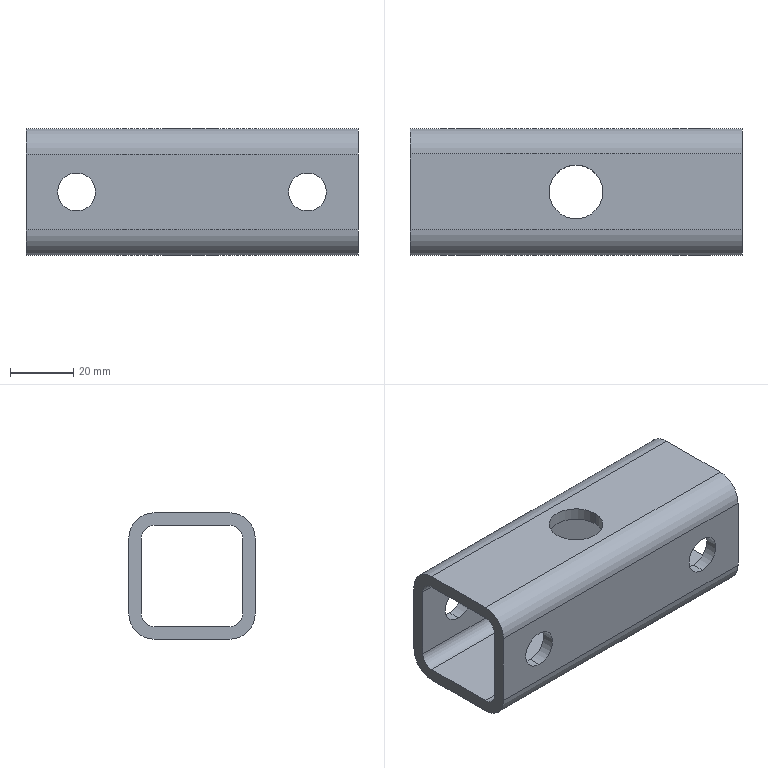Part | SolidWorks | features HoleWzd 1, ICE 1, WeldMemberFeat 1, WeldmentFeature 1 | 1 solid | 30 faces | box 105 x 40 x 40 mm | volume 52528 mm3 | cylinder 20 | plane 10 | commonest cylinder face diameters 12 x8 8 x4 16 x4 17 x4
STEP:
#1=CARTESIAN_POINT('',(44.,0.,20.));
#2=VERTEX_POINT('',#1);
#3=CARTESIAN_POINT('',(61.,0.,20.));
#4=VERTEX_POINT('',#3);
#5=CARTESIAN_POINT('',(52.5,0.,20.));
#6=DIRECTION('',(0.,0.,1.));
#7=DIRECTION('',(-1.,0.,0.));
#8=AXIS2_PLACEMENT_3D('',#5,#6,#7);
#9=CIRCLE('',#8,8.5);
#10=EDGE_CURVE('',#2,#4,#9,.T.);
#11=ORIENTED_EDGE('',*,*,#10,.T.);
#12=CARTESIAN_POINT('',(61.,0.,16.));
#13=VERTEX_POINT('',#12);
#14=CARTESIAN_POINT('',(61.,0.,44.042));
#15=DIRECTION('',(0.,0.,-1.));
#16=VECTOR('',#15,1000.);
#17=LINE('',#14,#16);
#18=EDGE_CURVE('',#4,#13,#17,.T.);
#19=ORIENTED_EDGE('',*,*,#18,.T.);
#20=CARTESIAN_POINT('',(44.,0.,16.));
#21=VERTEX_POINT('',#20);
#22=CARTESIAN_POINT('',(52.5,0.,16.));
#23=DIRECTION('',(0.,0.,-1.));
#24=DIRECTION('',(-1.,0.,0.));
#25=AXIS2_PLACEMENT_3D('',#22,#23,#24);
#26=CIRCLE('',#25,8.5);
#27=EDGE_CURVE('',#13,#21,#26,.T.);
#28=ORIENTED_EDGE('',*,*,#27,.T.);
#29=CARTESIAN_POINT('',(44.,0.,44.042));
#30=DIRECTION('',(0.,0.,-1.));
#31=VECTOR('',#30,1000.);
#32=LINE('',#29,#31);
#33=EDGE_CURVE('',#2,#21,#32,.T.);
#34=ORIENTED_EDGE('',*,*,#33,.F.);
#35=EDGE_LOOP('',(#11,#19,#28,#34));
#36=FACE_OUTER_BOUND('',#35,.T.);
#37=CARTESIAN_POINT('',(52.5,0.,44.042));
#38=DIRECTION('',(0.,0.,-1.));
#39=DIRECTION('',(-1.,0.,0.));
#40=AXIS2_PLACEMENT_3D('',#37,#38,#39);
#41=CYLINDRICAL_SURFACE('',#40,8.5);
#42=ADVANCED_FACE('',(#36),#41,.F.);
#43=CARTESIAN_POINT('',(44.,0.,-16.));
#44=VERTEX_POINT('',#43);
#45=CARTESIAN_POINT('',(61.,0.,-16.));
#46=VERTEX_POINT('',#45);
#47=CARTESIAN_POINT('',(52.5,0.,-16.));
#48=DIRECTION('',(0.,0.,1.));
#49=DIRECTION('',(1.,0.,0.));
#50=AXIS2_PLACEMENT_3D('',#47,#48,#49);
#51=CIRCLE('',#50,8.5);
#52=EDGE_CURVE('',#44,#46,#51,.T.);
#53=ORIENTED_EDGE('',*,*,#52,.T.);
#54=CARTESIAN_POINT('',(61.,0.,-20.));
#55=VERTEX_POINT('',#54);
#56=CARTESIAN_POINT('',(61.,0.,44.042));
#57=DIRECTION('',(0.,0.,-1.));
#58=VECTOR('',#57,1000.);
#59=LINE('',#56,#58);
#60=EDGE_CURVE('',#46,#55,#59,.T.);
#61=ORIENTED_EDGE('',*,*,#60,.T.);
#62=CARTESIAN_POINT('',(44.,0.,-20.));
#63=VERTEX_POINT('',#62);
#64=CARTESIAN_POINT('',(52.5,0.,-20.));
#65=DIRECTION('',(0.,0.,-1.));
#66=DIRECTION('',(-1.,0.,0.));
#67=AXIS2_PLACEMENT_3D('',#64,#65,#66);
#68=CIRCLE('',#67,8.5);
#69=EDGE_CURVE('',#55,#63,#68,.T.);
#70=ORIENTED_EDGE('',*,*,#69,.T.);
#71=CARTESIAN_POINT('',(44.,0.,44.042));
#72=DIRECTION('',(0.,0.,-1.));
#73=VECTOR('',#72,1000.);
#74=LINE('',#71,#73);
#75=EDGE_CURVE('',#44,#63,#74,.T.);
#76=ORIENTED_EDGE('',*,*,#75,.F.);
#77=EDGE_LOOP('',(#53,#61,#70,#76));
#78=FACE_OUTER_BOUND('',#77,.T.);
#79=CARTESIAN_POINT('',(52.5,0.,44.042));
#80=DIRECTION('',(0.,0.,-1.));
#81=DIRECTION('',(-1.,0.,0.));
#82=AXIS2_PLACEMENT_3D('',#79,#80,#81);
#83=CYLINDRICAL_SURFACE('',#82,8.5);
#84=ADVANCED_FACE('',(#78),#83,.F.);
#85=CARTESIAN_POINT('',(16.,-20.,-6.));
#86=VERTEX_POINT('',#85);
#87=CARTESIAN_POINT('',(16.,-20.,6.));
#88=VERTEX_POINT('',#87);
#89=CARTESIAN_POINT('',(16.,-20.,0.));
#90=DIRECTION('',(0.,1.,0.));
#91=DIRECTION('',(0.,0.,1.));
#92=AXIS2_PLACEMENT_3D('',#89,#90,#91);
#93=CIRCLE('',#92,6.);
#94=EDGE_CURVE('',#86,#88,#93,.T.);
#95=ORIENTED_EDGE('',*,*,#94,.F.);
#96=CARTESIAN_POINT('',(16.,-16.,-6.));
#97=VERTEX_POINT('',#96);
#98=CARTESIAN_POINT('',(16.,20.,-6.));
#99=DIRECTION('',(0.,1.,0.));
#100=VECTOR('',#99,1000.);
#101=LINE('',#98,#100);
#102=EDGE_CURVE('',#86,#97,#101,.T.);
#103=ORIENTED_EDGE('',*,*,#102,.T.);
#104=CARTESIAN_POINT('',(16.,-16.,6.));
#105=VERTEX_POINT('',#104);
#106=CARTESIAN_POINT('',(16.,-16.,0.));
#107=DIRECTION('',(0.,1.,0.));
#108=DIRECTION('',(0.,0.,1.));
#109=AXIS2_PLACEMENT_3D('',#106,#107,#108);
#110=CIRCLE('',#109,6.);
#111=EDGE_CURVE('',#97,#105,#110,.T.);
#112=ORIENTED_EDGE('',*,*,#111,.T.);
#113=CARTESIAN_POINT('',(16.,20.,6.));
#114=DIRECTION('',(0.,1.,0.));
#115=VECTOR('',#114,1000.);
#116=LINE('',#113,#115);
#117=EDGE_CURVE('',#88,#105,#116,.T.);
#118=ORIENTED_EDGE('',*,*,#117,.F.);
#119=EDGE_LOOP('',(#95,#103,#112,#118));
#120=FACE_OUTER_BOUND('',#119,.T.);
#121=CARTESIAN_POINT('',(16.,20.,0.));
#122=DIRECTION('',(0.,1.,0.));
#123=DIRECTION('',(0.,0.,1.));
#124=AXIS2_PLACEMENT_3D('',#121,#122,#123);
#125=CYLINDRICAL_SURFACE('',#124,6.);
#126=ADVANCED_FACE('',(#120),#125,.F.);
#127=CARTESIAN_POINT('',(16.,16.,6.));
#128=VERTEX_POINT('',#127);
#129=CARTESIAN_POINT('',(16.,16.,-6.));
#130=VERTEX_POINT('',#129);
#131=CARTESIAN_POINT('',(16.,16.,0.));
#132=DIRECTION('',(0.,-1.,0.));
#133=DIRECTION('',(0.,0.,-1.));
#134=AXIS2_PLACEMENT_3D('',#131,#132,#133);
#135=CIRCLE('',#134,6.);
#136=EDGE_CURVE('',#128,#130,#135,.T.);
#137=ORIENTED_EDGE('',*,*,#136,.T.);
#138=CARTESIAN_POINT('',(16.,20.,-6.));
#139=VERTEX_POINT('',#138);
#140=CARTESIAN_POINT('',(16.,20.,-6.));
#141=DIRECTION('',(0.,1.,0.));
#142=VECTOR('',#141,1000.);
#143=LINE('',#140,#142);
#144=EDGE_CURVE('',#130,#139,#143,.T.);
#145=ORIENTED_EDGE('',*,*,#144,.T.);
#146=CARTESIAN_POINT('',(16.,20.,6.));
#147=VERTEX_POINT('',#146);
#148=CARTESIAN_POINT('',(16.,20.,0.));
#149=DIRECTION('',(0.,1.,0.));
#150=DIRECTION('',(0.,0.,1.));
#151=AXIS2_PLACEMENT_3D('',#148,#149,#150);
#152=CIRCLE('',#151,6.);
#153=EDGE_CURVE('',#139,#147,#152,.T.);
#154=ORIENTED_EDGE('',*,*,#153,.T.);
#155=CARTESIAN_POINT('',(16.,20.,6.));
#156=DIRECTION('',(0.,1.,0.));
#157=VECTOR('',#156,1000.);
#158=LINE('',#155,#157);
#159=EDGE_CURVE('',#128,#147,#158,.T.);
#160=ORIENTED_EDGE('',*,*,#159,.F.);
#161=EDGE_LOOP('',(#137,#145,#154,#160));
#162=FACE_OUTER_BOUND('',#161,.T.);
#163=CARTESIAN_POINT('',(16.,20.,0.));
#164=DIRECTION('',(0.,1.,0.));
#165=DIRECTION('',(0.,0.,1.));
#166=AXIS2_PLACEMENT_3D('',#163,#164,#165);
#167=CYLINDRICAL_SURFACE('',#166,6.);
#168=ADVANCED_FACE('',(#162),#167,.F.);
#169=CARTESIAN_POINT('',(89.,-20.,-6.));
#170=VERTEX_POINT('',#169);
#171=CARTESIAN_POINT('',(89.,-20.,6.));
#172=VERTEX_POINT('',#171);
#173=CARTESIAN_POINT('',(89.,-20.,0.));
#174=DIRECTION('',(0.,1.,0.));
#175=DIRECTION('',(0.,0.,1.));
#176=AXIS2_PLACEMENT_3D('',#173,#174,#175);
#177=CIRCLE('',#176,6.);
#178=EDGE_CURVE('',#170,#172,#177,.T.);
#179=ORIENTED_EDGE('',*,*,#178,.F.);
#180=CARTESIAN_POINT('',(89.,-16.,-6.));
#181=VERTEX_POINT('',#180);
#182=CARTESIAN_POINT('',(89.,20.,-6.));
#183=DIRECTION('',(0.,1.,0.));
#184=VECTOR('',#183,1000.);
#185=LINE('',#182,#184);
#186=EDGE_CURVE('',#170,#181,#185,.T.);
#187=ORIENTED_EDGE('',*,*,#186,.T.);
#188=CARTESIAN_POINT('',(89.,-16.,6.));
#189=VERTEX_POINT('',#188);
#190=CARTESIAN_POINT('',(89.,-16.,0.));
#191=DIRECTION('',(0.,1.,0.));
#192=DIRECTION('',(0.,0.,1.));
#193=AXIS2_PLACEMENT_3D('',#190,#191,#192);
#194=CIRCLE('',#193,6.);
#195=EDGE_CURVE('',#181,#189,#194,.T.);
#196=ORIENTED_EDGE('',*,*,#195,.T.);
#197=CARTESIAN_POINT('',(89.,20.,6.));
#198=DIRECTION('',(0.,1.,0.));
#199=VECTOR('',#198,1000.);
#200=LINE('',#197,#199);
#201=EDGE_CURVE('',#172,#189,#200,.T.);
#202=ORIENTED_EDGE('',*,*,#201,.F.);
#203=EDGE_LOOP('',(#179,#187,#196,#202));
#204=FACE_OUTER_BOUND('',#203,.T.);
#205=CARTESIAN_POINT('',(89.,20.,0.));
#206=DIRECTION('',(0.,1.,0.));
#207=DIRECTION('',(0.,0.,1.));
#208=AXIS2_PLACEMENT_3D('',#205,#206,#207);
#209=CYLINDRICAL_SURFACE('',#208,6.);
#210=ADVANCED_FACE('',(#204),#209,.F.);
#211=CARTESIAN_POINT('',(89.,16.,6.));
#212=VERTEX_POINT('',#211);
#213=CARTESIAN_POINT('',(89.,16.,-6.));
#214=VERTEX_POINT('',#213);
#215=CARTESIAN_POINT('',(89.,16.,0.));
#216=DIRECTION('',(0.,-1.,0.));
#217=DIRECTION('',(0.,0.,-1.));
#218=AXIS2_PLACEMENT_3D('',#215,#216,#217);
#219=CIRCLE('',#218,6.);
#220=EDGE_CURVE('',#212,#214,#219,.T.);
#221=ORIENTED_EDGE('',*,*,#220,.T.);
#222=CARTESIAN_POINT('',(89.,20.,-6.));
#223=VERTEX_POINT('',#222);
#224=CARTESIAN_POINT('',(89.,20.,-6.));
#225=DIRECTION('',(0.,1.,0.));
#226=VECTOR('',#225,1000.);
#227=LINE('',#224,#226);
#228=EDGE_CURVE('',#214,#223,#227,.T.);
#229=ORIENTED_EDGE('',*,*,#228,.T.);
#230=CARTESIAN_POINT('',(89.,20.,6.));
#231=VERTEX_POINT('',#230);
#232=CARTESIAN_POINT('',(89.,20.,0.));
#233=DIRECTION('',(0.,1.,0.));
#234=DIRECTION('',(0.,0.,1.));
#235=AXIS2_PLACEMENT_3D('',#232,#233,#234);
#236=CIRCLE('',#235,6.);
#237=EDGE_CURVE('',#223,#231,#236,.T.);
#238=ORIENTED_EDGE('',*,*,#237,.T.);
#239=CARTESIAN_POINT('',(89.,20.,6.));
#240=DIRECTION('',(0.,1.,0.));
#241=VECTOR('',#240,1000.);
#242=LINE('',#239,#241);
#243=EDGE_CURVE('',#212,#231,#242,.T.);
#244=ORIENTED_EDGE('',*,*,#243,.F.);
#245=EDGE_LOOP('',(#221,#229,#238,#244));
#246=FACE_OUTER_BOUND('',#245,.T.);
#247=CARTESIAN_POINT('',(89.,20.,0.));
#248=DIRECTION('',(0.,1.,0.));
#249=DIRECTION('',(0.,0.,1.));
#250=AXIS2_PLACEMENT_3D('',#247,#248,#249);
#251=CYLINDRICAL_SURFACE('',#250,6.);
#252=ADVANCED_FACE('',(#246),#251,.F.);
#253=CARTESIAN_POINT('',(0.,20.,12.));
#254=VERTEX_POINT('',#253);
#255=CARTESIAN_POINT('',(0.,12.,20.));
#256=VERTEX_POINT('',#255);
#257=CARTESIAN_POINT('',(0.,12.,12.));
#258=DIRECTION('',(1.,0.,0.));
#259=DIRECTION('',(0.,0.,-1.));
#260=AXIS2_PLACEMENT_3D('',#257,#258,#259);
#261=CIRCLE('',#260,8.);
#262=EDGE_CURVE('',#254,#256,#261,.T.);
#263=ORIENTED_EDGE('',*,*,#262,.T.);
#264=CARTESIAN_POINT('',(105.,12.,20.));
#265=VERTEX_POINT('',#264);
#266=CARTESIAN_POINT('',(105.,12.,20.));
#267=DIRECTION('',(-1.,0.,0.));
#268=VECTOR('',#267,1000.);
#269=LINE('',#266,#268);
#270=EDGE_CURVE('',#265,#256,#269,.T.);
#271=ORIENTED_EDGE('',*,*,#270,.F.);
#272=CARTESIAN_POINT('',(105.,20.,12.));
#273=VERTEX_POINT('',#272);
#274=CARTESIAN_POINT('',(105.,12.,12.));
#275=DIRECTION('',(1.,0.,0.));
#276=DIRECTION('',(0.,0.,-1.));
#277=AXIS2_PLACEMENT_3D('',#274,#275,#276);
#278=CIRCLE('',#277,8.);
#279=EDGE_CURVE('',#273,#265,#278,.T.);
#280=ORIENTED_EDGE('',*,*,#279,.F.);
#281=CARTESIAN_POINT('',(105.,20.,12.));
#282=DIRECTION('',(-1.,0.,0.));
#283=VECTOR('',#282,1000.);
#284=LINE('',#281,#283);
#285=EDGE_CURVE('',#273,#254,#284,.T.);
#286=ORIENTED_EDGE('',*,*,#285,.T.);
#287=EDGE_LOOP('',(#263,#271,#280,#286));
#288=FACE_OUTER_BOUND('',#287,.T.);
#289=CARTESIAN_POINT('',(105.,12.,12.));
#290=DIRECTION('',(-1.,0.,0.));
#291=DIRECTION('',(0.,0.,1.));
#292=AXIS2_PLACEMENT_3D('',#289,#290,#291);
#293=CYLINDRICAL_SURFACE('',#292,8.);
#294=ADVANCED_FACE('',(#288),#293,.T.);
#295=ORIENTED_EDGE('',*,*,#10,.F.);
#296=CARTESIAN_POINT('',(52.5,0.,20.));
#297=DIRECTION('',(0.,0.,1.));
#298=DIRECTION('',(-1.,0.,0.));
#299=AXIS2_PLACEMENT_3D('',#296,#297,#298);
#300=CIRCLE('',#299,8.5);
#301=EDGE_CURVE('',#4,#2,#300,.T.);
#302=ORIENTED_EDGE('',*,*,#301,.F.);
#303=EDGE_LOOP('',(#295,#302));
#304=FACE_BOUND('',#303,.T.);
#305=CARTESIAN_POINT('',(0.,-12.,20.));
#306=VERTEX_POINT('',#305);
#307=CARTESIAN_POINT('',(0.,12.,20.));
#308=DIRECTION('',(0.,-1.,0.));
#309=VECTOR('',#308,1000.);
#310=LINE('',#307,#309);
#311=EDGE_CURVE('',#256,#306,#310,.T.);
#312=ORIENTED_EDGE('',*,*,#311,.T.);
#313=CARTESIAN_POINT('',(105.,-12.,20.));
#314=VERTEX_POINT('',#313);
#315=CARTESIAN_POINT('',(105.,-12.,20.));
#316=DIRECTION('',(-1.,0.,0.));
#317=VECTOR('',#316,1000.);
#318=LINE('',#315,#317);
#319=EDGE_CURVE('',#314,#306,#318,.T.);
#320=ORIENTED_EDGE('',*,*,#319,.F.);
#321=CARTESIAN_POINT('',(105.,12.,20.));
#322=DIRECTION('',(0.,-1.,0.));
#323=VECTOR('',#322,1000.);
#324=LINE('',#321,#323);
#325=EDGE_CURVE('',#265,#314,#324,.T.);
#326=ORIENTED_EDGE('',*,*,#325,.F.);
#327=ORIENTED_EDGE('',*,*,#270,.T.);
#328=EDGE_LOOP('',(#312,#320,#326,#327));
#329=FACE_OUTER_BOUND('',#328,.T.);
#330=CARTESIAN_POINT('',(105.,12.,20.));
#331=DIRECTION('',(0.,0.,-1.));
#332=DIRECTION('',(-1.,0.,0.));
#333=AXIS2_PLACEMENT_3D('',#330,#331,#332);
#334=PLANE('',#333);
#335=ADVANCED_FACE('',(#304,#329),#334,.F.);
#336=CARTESIAN_POINT('',(0.,-20.,12.));
#337=VERTEX_POINT('',#336);
#338=CARTESIAN_POINT('',(0.,-12.,12.));
#339=DIRECTION('',(1.,0.,0.));
#340=DIRECTION('',(0.,0.,-1.));
#341=AXIS2_PLACEMENT_3D('',#338,#339,#340);
#342=CIRCLE('',#341,8.);
#343=EDGE_CURVE('',#306,#337,#342,.T.);
#344=ORIENTED_EDGE('',*,*,#343,.T.);
#345=CARTESIAN_POINT('',(105.,-20.,12.));
#346=VERTEX_POINT('',#345);
#347=CARTESIAN_POINT('',(105.,-20.,12.));
#348=DIRECTION('',(-1.,0.,0.));
#349=VECTOR('',#348,1000.);
#350=LINE('',#347,#349);
#351=EDGE_CURVE('',#346,#337,#350,.T.);
#352=ORIENTED_EDGE('',*,*,#351,.F.);
#353=CARTESIAN_POINT('',(105.,-12.,12.));
#354=DIRECTION('',(1.,0.,0.));
#355=DIRECTION('',(0.,0.,-1.));
#356=AXIS2_PLACEMENT_3D('',#353,#354,#355);
#357=CIRCLE('',#356,8.);
#358=EDGE_CURVE('',#314,#346,#357,.T.);
#359=ORIENTED_EDGE('',*,*,#358,.F.);
#360=ORIENTED_EDGE('',*,*,#319,.T.);
#361=EDGE_LOOP('',(#344,#352,#359,#360));
#362=FACE_OUTER_BOUND('',#361,.T.);
#363=CARTESIAN_POINT('',(105.,-12.,12.));
#364=DIRECTION('',(-1.,0.,0.));
#365=DIRECTION('',(0.,0.,1.));
#366=AXIS2_PLACEMENT_3D('',#363,#364,#365);
#367=CYLINDRICAL_SURFACE('',#366,8.);
#368=ADVANCED_FACE('',(#362),#367,.T.);
#369=CARTESIAN_POINT('',(16.,-20.,0.));
#370=DIRECTION('',(0.,1.,0.));
#371=DIRECTION('',(0.,0.,1.));
#372=AXIS2_PLACEMENT_3D('',#369,#370,#371);
#373=CIRCLE('',#372,6.);
#374=EDGE_CURVE('',#88,#86,#373,.T.);
#375=ORIENTED_EDGE('',*,*,#374,.T.);
#376=ORIENTED_EDGE('',*,*,#94,.T.);
#377=EDGE_LOOP('',(#375,#376));
#378=FACE_BOUND('',#377,.T.);
#379=CARTESIAN_POINT('',(89.,-20.,0.));
#380=DIRECTION('',(0.,1.,0.));
#381=DIRECTION('',(0.,0.,1.));
#382=AXIS2_PLACEMENT_3D('',#379,#380,#381);
#383=CIRCLE('',#382,6.);
#384=EDGE_CURVE('',#172,#170,#383,.T.);
#385=ORIENTED_EDGE('',*,*,#384,.T.);
#386=ORIENTED_EDGE('',*,*,#178,.T.);
#387=EDGE_LOOP('',(#385,#386));
#388=FACE_BOUND('',#387,.T.);
#389=CARTESIAN_POINT('',(0.,-20.,-12.));
#390=VERTEX_POINT('',#389);
#391=CARTESIAN_POINT('',(0.,-20.,-12.));
#392=DIRECTION('',(0.,0.,-1.));
#393=VECTOR('',#392,1000.);
#394=LINE('',#391,#393);
#395=EDGE_CURVE('',#337,#390,#394,.T.);
#396=ORIENTED_EDGE('',*,*,#395,.T.);
#397=CARTESIAN_POINT('',(105.,-20.,-12.));
#398=VERTEX_POINT('',#397);
#399=CARTESIAN_POINT('',(105.,-20.,-12.));
#400=DIRECTION('',(-1.,0.,0.));
#401=VECTOR('',#400,1000.);
#402=LINE('',#399,#401);
#403=EDGE_CURVE('',#398,#390,#402,.T.);
#404=ORIENTED_EDGE('',*,*,#403,.F.);
#405=CARTESIAN_POINT('',(105.,-20.,-12.));
#406=DIRECTION('',(0.,0.,-1.));
#407=VECTOR('',#406,1000.);
#408=LINE('',#405,#407);
#409=EDGE_CURVE('',#346,#398,#408,.T.);
#410=ORIENTED_EDGE('',*,*,#409,.F.);
#411=ORIENTED_EDGE('',*,*,#351,.T.);
#412=EDGE_LOOP('',(#396,#404,#410,#411));
#413=FACE_OUTER_BOUND('',#412,.T.);
#414=CARTESIAN_POINT('',(105.,-20.,-12.));
#415=DIRECTION('',(0.,1.,0.));
#416=DIRECTION('',(0.,0.,1.));
#417=AXIS2_PLACEMENT_3D('',#414,#415,#416);
#418=PLANE('',#417);
#419=ADVANCED_FACE('',(#378,#388,#413),#418,.F.);
#420=CARTESIAN_POINT('',(0.,-12.,-20.));
#421=VERTEX_POINT('',#420);
#422=CARTESIAN_POINT('',(0.,-12.,-12.));
#423=DIRECTION('',(1.,0.,0.));
#424=DIRECTION('',(0.,0.,-1.));
#425=AXIS2_PLACEMENT_3D('',#422,#423,#424);
#426=CIRCLE('',#425,8.);
#427=EDGE_CURVE('',#390,#421,#426,.T.);
#428=ORIENTED_EDGE('',*,*,#427,.T.);
#429=CARTESIAN_POINT('',(105.,-12.,-20.));
#430=VERTEX_POINT('',#429);
#431=CARTESIAN_POINT('',(105.,-12.,-20.));
#432=DIRECTION('',(-1.,0.,0.));
#433=VECTOR('',#432,1000.);
#434=LINE('',#431,#433);
#435=EDGE_CURVE('',#430,#421,#434,.T.);
#436=ORIENTED_EDGE('',*,*,#435,.F.);
#437=CARTESIAN_POINT('',(105.,-12.,-12.));
#438=DIRECTION('',(1.,0.,0.));
#439=DIRECTION('',(0.,0.,-1.));
#440=AXIS2_PLACEMENT_3D('',#437,#438,#439);
#441=CIRCLE('',#440,8.);
#442=EDGE_CURVE('',#398,#430,#441,.T.);
#443=ORIENTED_EDGE('',*,*,#442,.F.);
#444=ORIENTED_EDGE('',*,*,#403,.T.);
#445=EDGE_LOOP('',(#428,#436,#443,#444));
#446=FACE_OUTER_BOUND('',#445,.T.);
#447=CARTESIAN_POINT('',(105.,-12.,-12.));
#448=DIRECTION('',(-1.,0.,0.));
#449=DIRECTION('',(0.,0.,1.));
#450=AXIS2_PLACEMENT_3D('',#447,#448,#449);
#451=CYLINDRICAL_SURFACE('',#450,8.);
#452=ADVANCED_FACE('',(#446),#451,.T.);
#453=CARTESIAN_POINT('',(52.5,0.,-20.));
#454=DIRECTION('',(0.,0.,-1.));
#455=DIRECTION('',(-1.,0.,0.));
#456=AXIS2_PLACEMENT_3D('',#453,#454,#455);
#457=CIRCLE('',#456,8.5);
#458=EDGE_CURVE('',#63,#55,#457,.T.);
#459=ORIENTED_EDGE('',*,*,#458,.F.);
#460=ORIENTED_EDGE('',*,*,#69,.F.);
#461=EDGE_LOOP('',(#459,#460));
#462=FACE_BOUND('',#461,.T.);
#463=CARTESIAN_POINT('',(0.,12.,-20.));
#464=VERTEX_POINT('',#463);
#465=CARTESIAN_POINT('',(0.,-12.,-20.));
#466=DIRECTION('',(0.,1.,0.));
#467=VECTOR('',#466,1000.);
#468=LINE('',#465,#467);
#469=EDGE_CURVE('',#421,#464,#468,.T.);
#470=ORIENTED_EDGE('',*,*,#469,.T.);
#471=CARTESIAN_POINT('',(105.,12.,-20.));
#472=VERTEX_POINT('',#471);
#473=CARTESIAN_POINT('',(105.,12.,-20.));
#474=DIRECTION('',(-1.,0.,0.));
#475=VECTOR('',#474,1000.);
#476=LINE('',#473,#475);
#477=EDGE_CURVE('',#472,#464,#476,.T.);
#478=ORIENTED_EDGE('',*,*,#477,.F.);
#479=CARTESIAN_POINT('',(105.,-12.,-20.));
#480=DIRECTION('',(0.,1.,0.));
#481=VECTOR('',#480,1000.);
#482=LINE('',#479,#481);
#483=EDGE_CURVE('',#430,#472,#482,.T.);
#484=ORIENTED_EDGE('',*,*,#483,.F.);
#485=ORIENTED_EDGE('',*,*,#435,.T.);
#486=EDGE_LOOP('',(#470,#478,#484,#485));
#487=FACE_OUTER_BOUND('',#486,.T.);
#488=CARTESIAN_POINT('',(105.,-12.,-20.));
#489=DIRECTION('',(0.,0.,1.));
#490=DIRECTION('',(1.,0.,0.));
#491=AXIS2_PLACEMENT_3D('',#488,#489,#490);
#492=PLANE('',#491);
#493=ADVANCED_FACE('',(#462,#487),#492,.F.);
#494=CARTESIAN_POINT('',(0.,20.,-12.));
#495=VERTEX_POINT('',#494);
#496=CARTESIAN_POINT('',(0.,12.,-12.));
#497=DIRECTION('',(1.,0.,0.));
#498=DIRECTION('',(0.,0.,-1.));
#499=AXIS2_PLACEMENT_3D('',#496,#497,#498);
#500=CIRCLE('',#499,8.);
#501=EDGE_CURVE('',#464,#495,#500,.T.);
#502=ORIENTED_EDGE('',*,*,#501,.T.);
#503=CARTESIAN_POINT('',(105.,20.,-12.));
#504=VERTEX_POINT('',#503);
#505=CARTESIAN_POINT('',(105.,20.,-12.));
#506=DIRECTION('',(-1.,0.,0.));
#507=VECTOR('',#506,1000.);
#508=LINE('',#505,#507);
#509=EDGE_CURVE('',#504,#495,#508,.T.);
#510=ORIENTED_EDGE('',*,*,#509,.F.);
#511=CARTESIAN_POINT('',(105.,12.,-12.));
#512=DIRECTION('',(1.,0.,0.));
#513=DIRECTION('',(0.,0.,-1.));
#514=AXIS2_PLACEMENT_3D('',#511,#512,#513);
#515=CIRCLE('',#514,8.);
#516=EDGE_CURVE('',#472,#504,#515,.T.);
#517=ORIENTED_EDGE('',*,*,#516,.F.);
#518=ORIENTED_EDGE('',*,*,#477,.T.);
#519=EDGE_LOOP('',(#502,#510,#517,#518));
#520=FACE_OUTER_BOUND('',#519,.T.);
#521=CARTESIAN_POINT('',(105.,12.,-12.));
#522=DIRECTION('',(-1.,0.,0.));
#523=DIRECTION('',(0.,0.,1.));
#524=AXIS2_PLACEMENT_3D('',#521,#522,#523);
#525=CYLINDRICAL_SURFACE('',#524,8.);
#526=ADVANCED_FACE('',(#520),#525,.T.);
#527=CARTESIAN_POINT('',(0.,-12.,16.));
#528=VERTEX_POINT('',#527);
#529=CARTESIAN_POINT('',(0.,-16.,12.));
#530=VERTEX_POINT('',#529);
#531=CARTESIAN_POINT('',(0.,-12.,12.));
#532=DIRECTION('',(1.,0.,0.));
#533=DIRECTION('',(0.,0.,-1.));
#534=AXIS2_PLACEMENT_3D('',#531,#532,#533);
#535=CIRCLE('',#534,4.);
#536=EDGE_CURVE('',#528,#530,#535,.T.);
#537=ORIENTED_EDGE('',*,*,#536,.F.);
#538=CARTESIAN_POINT('',(105.,-12.,16.));
#539=VERTEX_POINT('',#538);
#540=CARTESIAN_POINT('',(105.,-12.,16.));
#541=DIRECTION('',(-1.,0.,0.));
#542=VECTOR('',#541,1000.);
#543=LINE('',#540,#542);
#544=EDGE_CURVE('',#539,#528,#543,.T.);
#545=ORIENTED_EDGE('',*,*,#544,.F.);
#546=CARTESIAN_POINT('',(105.,-16.,12.));
#547=VERTEX_POINT('',#546);
#548=CARTESIAN_POINT('',(105.,-12.,12.));
#549=DIRECTION('',(1.,0.,0.));
#550=DIRECTION('',(0.,0.,-1.));
#551=AXIS2_PLACEMENT_3D('',#548,#549,#550);
#552=CIRCLE('',#551,4.);
#553=EDGE_CURVE('',#539,#547,#552,.T.);
#554=ORIENTED_EDGE('',*,*,#553,.T.);
#555=CARTESIAN_POINT('',(105.,-16.,12.));
#556=DIRECTION('',(-1.,0.,0.));
#557=VECTOR('',#556,1000.);
#558=LINE('',#555,#557);
#559=EDGE_CURVE('',#547,#530,#558,.T.);
#560=ORIENTED_EDGE('',*,*,#559,.T.);
#561=EDGE_LOOP('',(#537,#545,#554,#560));
#562=FACE_OUTER_BOUND('',#561,.T.);
#563=CARTESIAN_POINT('',(105.,-12.,12.));
#564=DIRECTION('',(-1.,0.,0.));
#565=DIRECTION('',(0.,0.,1.));
#566=AXIS2_PLACEMENT_3D('',#563,#564,#565);
#567=CYLINDRICAL_SURFACE('',#566,4.);
#568=ADVANCED_FACE('',(#562),#567,.F.);
#569=CARTESIAN_POINT('',(52.5,0.,16.));
#570=DIRECTION('',(0.,0.,-1.));
#571=DIRECTION('',(-1.,0.,0.));
#572=AXIS2_PLACEMENT_3D('',#569,#570,#571);
#573=CIRCLE('',#572,8.5);
#574=EDGE_CURVE('',#21,#13,#573,.T.);
#575=ORIENTED_EDGE('',*,*,#574,.F.);
#576=ORIENTED_EDGE('',*,*,#27,.F.);
#577=EDGE_LOOP('',(#575,#576));
#578=FACE_BOUND('',#577,.T.);
#579=CARTESIAN_POINT('',(0.,12.,16.));
#580=VERTEX_POINT('',#579);
#581=CARTESIAN_POINT('',(0.,12.,16.));
#582=DIRECTION('',(0.,-1.,0.));
#583=VECTOR('',#582,1000.);
#584=LINE('',#581,#583);
#585=EDGE_CURVE('',#580,#528,#584,.T.);
#586=ORIENTED_EDGE('',*,*,#585,.F.);
#587=CARTESIAN_POINT('',(105.,12.,16.));
#588=VERTEX_POINT('',#587);
#589=CARTESIAN_POINT('',(105.,12.,16.));
#590=DIRECTION('',(-1.,0.,0.));
#591=VECTOR('',#590,1000.);
#592=LINE('',#589,#591);
#593=EDGE_CURVE('',#588,#580,#592,.T.);
#594=ORIENTED_EDGE('',*,*,#593,.F.);
#595=CARTESIAN_POINT('',(105.,12.,16.));
#596=DIRECTION('',(0.,-1.,0.));
#597=VECTOR('',#596,1000.);
#598=LINE('',#595,#597);
#599=EDGE_CURVE('',#588,#539,#598,.T.);
#600=ORIENTED_EDGE('',*,*,#599,.T.);
#601=ORIENTED_EDGE('',*,*,#544,.T.);
#602=EDGE_LOOP('',(#586,#594,#600,#601));
#603=FACE_OUTER_BOUND('',#602,.T.);
#604=CARTESIAN_POINT('',(105.,12.,16.));
#605=DIRECTION('',(0.,0.,-1.));
#606=DIRECTION('',(-1.,0.,0.));
#607=AXIS2_PLACEMENT_3D('',#604,#605,#606);
#608=PLANE('',#607);
#609=ADVANCED_FACE('',(#578,#603),#608,.T.);
#610=CARTESIAN_POINT('',(0.,16.,12.));
#611=VERTEX_POINT('',#610);
#612=CARTESIAN_POINT('',(0.,12.,12.));
#613=DIRECTION('',(1.,0.,0.));
#614=DIRECTION('',(0.,0.,-1.));
#615=AXIS2_PLACEMENT_3D('',#612,#613,#614);
#616=CIRCLE('',#615,4.);
#617=EDGE_CURVE('',#611,#580,#616,.T.);
#618=ORIENTED_EDGE('',*,*,#617,.F.);
#619=CARTESIAN_POINT('',(105.,16.,12.));
#620=VERTEX_POINT('',#619);
#621=CARTESIAN_POINT('',(105.,16.,12.));
#622=DIRECTION('',(-1.,0.,0.));
#623=VECTOR('',#622,1000.);
#624=LINE('',#621,#623);
#625=EDGE_CURVE('',#620,#611,#624,.T.);
#626=ORIENTED_EDGE('',*,*,#625,.F.);
#627=CARTESIAN_POINT('',(105.,12.,12.));
#628=DIRECTION('',(1.,0.,0.));
#629=DIRECTION('',(0.,0.,-1.));
#630=AXIS2_PLACEMENT_3D('',#627,#628,#629);
#631=CIRCLE('',#630,4.);
#632=EDGE_CURVE('',#620,#588,#631,.T.);
#633=ORIENTED_EDGE('',*,*,#632,.T.);
#634=ORIENTED_EDGE('',*,*,#593,.T.);
#635=EDGE_LOOP('',(#618,#626,#633,#634));
#636=FACE_OUTER_BOUND('',#635,.T.);
#637=CARTESIAN_POINT('',(105.,12.,12.));
#638=DIRECTION('',(-1.,0.,0.));
#639=DIRECTION('',(0.,0.,1.));
#640=AXIS2_PLACEMENT_3D('',#637,#638,#639);
#641=CYLINDRICAL_SURFACE('',#640,4.);
#642=ADVANCED_FACE('',(#636),#641,.F.);
#643=ORIENTED_EDGE('',*,*,#136,.F.);
#644=CARTESIAN_POINT('',(16.,16.,0.));
#645=DIRECTION('',(0.,-1.,0.));
#646=DIRECTION('',(0.,0.,-1.));
#647=AXIS2_PLACEMENT_3D('',#644,#645,#646);
#648=CIRCLE('',#647,6.);
#649=EDGE_CURVE('',#130,#128,#648,.T.);
#650=ORIENTED_EDGE('',*,*,#649,.F.);
#651=EDGE_LOOP('',(#643,#650));
#652=FACE_BOUND('',#651,.T.);
#653=ORIENTED_EDGE('',*,*,#220,.F.);
#654=CARTESIAN_POINT('',(89.,16.,0.));
#655=DIRECTION('',(0.,-1.,0.));
#656=DIRECTION('',(0.,0.,-1.));
#657=AXIS2_PLACEMENT_3D('',#654,#655,#656);
#658=CIRCLE('',#657,6.);
#659=EDGE_CURVE('',#214,#212,#658,.T.);
#660=ORIENTED_EDGE('',*,*,#659,.F.);
#661=EDGE_LOOP('',(#653,#660));
#662=FACE_BOUND('',#661,.T.);
#663=CARTESIAN_POINT('',(0.,16.,-12.));
#664=VERTEX_POINT('',#663);
#665=CARTESIAN_POINT('',(0.,16.,12.));
#666=DIRECTION('',(0.,0.,1.));
#667=VECTOR('',#666,1000.);
#668=LINE('',#665,#667);
#669=EDGE_CURVE('',#664,#611,#668,.T.);
#670=ORIENTED_EDGE('',*,*,#669,.F.);
#671=CARTESIAN_POINT('',(105.,16.,-12.));
#672=VERTEX_POINT('',#671);
#673=CARTESIAN_POINT('',(105.,16.,-12.));
#674=DIRECTION('',(-1.,0.,0.));
#675=VECTOR('',#674,1000.);
#676=LINE('',#673,#675);
#677=EDGE_CURVE('',#672,#664,#676,.T.);
#678=ORIENTED_EDGE('',*,*,#677,.F.);
#679=CARTESIAN_POINT('',(105.,16.,12.));
#680=DIRECTION('',(0.,0.,1.));
#681=VECTOR('',#680,1000.);
#682=LINE('',#679,#681);
#683=EDGE_CURVE('',#672,#620,#682,.T.);
#684=ORIENTED_EDGE('',*,*,#683,.T.);
#685=ORIENTED_EDGE('',*,*,#625,.T.);
#686=EDGE_LOOP('',(#670,#678,#684,#685));
#687=FACE_OUTER_BOUND('',#686,.T.);
#688=CARTESIAN_POINT('',(105.,16.,12.));
#689=DIRECTION('',(0.,-1.,0.));
#690=DIRECTION('',(0.,0.,-1.));
#691=AXIS2_PLACEMENT_3D('',#688,#689,#690);
#692=PLANE('',#691);
#693=ADVANCED_FACE('',(#652,#662,#687),#692,.T.);
#694=CARTESIAN_POINT('',(0.,12.,-16.));
#695=VERTEX_POINT('',#694);
#696=CARTESIAN_POINT('',(0.,12.,-12.));
#697=DIRECTION('',(1.,0.,0.));
#698=DIRECTION('',(0.,0.,-1.));
#699=AXIS2_PLACEMENT_3D('',#696,#697,#698);
#700=CIRCLE('',#699,4.);
#701=EDGE_CURVE('',#695,#664,#700,.T.);
#702=ORIENTED_EDGE('',*,*,#701,.F.);
#703=CARTESIAN_POINT('',(105.,12.,-16.));
#704=VERTEX_POINT('',#703);
#705=CARTESIAN_POINT('',(105.,12.,-16.));
#706=DIRECTION('',(-1.,0.,0.));
#707=VECTOR('',#706,1000.);
#708=LINE('',#705,#707);
#709=EDGE_CURVE('',#704,#695,#708,.T.);
#710=ORIENTED_EDGE('',*,*,#709,.F.);
#711=CARTESIAN_POINT('',(105.,12.,-12.));
#712=DIRECTION('',(1.,0.,0.));
#713=DIRECTION('',(0.,0.,-1.));
#714=AXIS2_PLACEMENT_3D('',#711,#712,#713);
#715=CIRCLE('',#714,4.);
#716=EDGE_CURVE('',#704,#672,#715,.T.);
#717=ORIENTED_EDGE('',*,*,#716,.T.);
#718=ORIENTED_EDGE('',*,*,#677,.T.);
#719=EDGE_LOOP('',(#702,#710,#717,#718));
#720=FACE_OUTER_BOUND('',#719,.T.);
#721=CARTESIAN_POINT('',(105.,12.,-12.));
#722=DIRECTION('',(-1.,0.,0.));
#723=DIRECTION('',(0.,0.,1.));
#724=AXIS2_PLACEMENT_3D('',#721,#722,#723);
#725=CYLINDRICAL_SURFACE('',#724,4.);
#726=ADVANCED_FACE('',(#720),#725,.F.);
#727=ORIENTED_EDGE('',*,*,#52,.F.);
#728=CARTESIAN_POINT('',(52.5,0.,-16.));
#729=DIRECTION('',(0.,0.,1.));
#730=DIRECTION('',(1.,0.,0.));
#731=AXIS2_PLACEMENT_3D('',#728,#729,#730);
#732=CIRCLE('',#731,8.5);
#733=EDGE_CURVE('',#46,#44,#732,.T.);
#734=ORIENTED_EDGE('',*,*,#733,.F.);
#735=EDGE_LOOP('',(#727,#734));
#736=FACE_BOUND('',#735,.T.);
#737=CARTESIAN_POINT('',(0.,-12.,-16.));
#738=VERTEX_POINT('',#737);
#739=CARTESIAN_POINT('',(0.,-12.,-16.));
#740=DIRECTION('',(0.,1.,0.));
#741=VECTOR('',#740,1000.);
#742=LINE('',#739,#741);
#743=EDGE_CURVE('',#738,#695,#742,.T.);
#744=ORIENTED_EDGE('',*,*,#743,.F.);
#745=CARTESIAN_POINT('',(105.,-12.,-16.));
#746=VERTEX_POINT('',#745);
#747=CARTESIAN_POINT('',(105.,-12.,-16.));
#748=DIRECTION('',(-1.,0.,0.));
#749=VECTOR('',#748,1000.);
#750=LINE('',#747,#749);
#751=EDGE_CURVE('',#746,#738,#750,.T.);
#752=ORIENTED_EDGE('',*,*,#751,.F.);
#753=CARTESIAN_POINT('',(105.,-12.,-16.));
#754=DIRECTION('',(0.,1.,0.));
#755=VECTOR('',#754,1000.);
#756=LINE('',#753,#755);
#757=EDGE_CURVE('',#746,#704,#756,.T.);
#758=ORIENTED_EDGE('',*,*,#757,.T.);
#759=ORIENTED_EDGE('',*,*,#709,.T.);
#760=EDGE_LOOP('',(#744,#752,#758,#759));
#761=FACE_OUTER_BOUND('',#760,.T.);
#762=CARTESIAN_POINT('',(105.,-12.,-16.));
#763=DIRECTION('',(0.,0.,1.));
#764=DIRECTION('',(1.,0.,0.));
#765=AXIS2_PLACEMENT_3D('',#762,#763,#764);
#766=PLANE('',#765);
#767=ADVANCED_FACE('',(#736,#761),#766,.T.);
#768=CARTESIAN_POINT('',(0.,-16.,-12.));
#769=VERTEX_POINT('',#768);
#770=CARTESIAN_POINT('',(0.,-12.,-12.));
#771=DIRECTION('',(1.,0.,0.));
#772=DIRECTION('',(0.,0.,-1.));
#773=AXIS2_PLACEMENT_3D('',#770,#771,#772);
#774=CIRCLE('',#773,4.);
#775=EDGE_CURVE('',#769,#738,#774,.T.);
#776=ORIENTED_EDGE('',*,*,#775,.F.);
#777=CARTESIAN_POINT('',(105.,-16.,-12.));
#778=VERTEX_POINT('',#777);
#779=CARTESIAN_POINT('',(105.,-16.,-12.));
#780=DIRECTION('',(-1.,0.,0.));
#781=VECTOR('',#780,1000.);
#782=LINE('',#779,#781);
#783=EDGE_CURVE('',#778,#769,#782,.T.);
#784=ORIENTED_EDGE('',*,*,#783,.F.);
#785=CARTESIAN_POINT('',(105.,-12.,-12.));
#786=DIRECTION('',(1.,0.,0.));
#787=DIRECTION('',(0.,0.,-1.));
#788=AXIS2_PLACEMENT_3D('',#785,#786,#787);
#789=CIRCLE('',#788,4.);
#790=EDGE_CURVE('',#778,#746,#789,.T.);
#791=ORIENTED_EDGE('',*,*,#790,.T.);
#792=ORIENTED_EDGE('',*,*,#751,.T.);
#793=EDGE_LOOP('',(#776,#784,#791,#792));
#794=FACE_OUTER_BOUND('',#793,.T.);
#795=CARTESIAN_POINT('',(105.,-12.,-12.));
#796=DIRECTION('',(-1.,0.,0.));
#797=DIRECTION('',(0.,0.,1.));
#798=AXIS2_PLACEMENT_3D('',#795,#796,#797);
#799=CYLINDRICAL_SURFACE('',#798,4.);
#800=ADVANCED_FACE('',(#794),#799,.F.);
#801=CARTESIAN_POINT('',(16.,-16.,0.));
#802=DIRECTION('',(0.,1.,0.));
#803=DIRECTION('',(0.,0.,1.));
#804=AXIS2_PLACEMENT_3D('',#801,#802,#803);
#805=CIRCLE('',#804,6.);
#806=EDGE_CURVE('',#105,#97,#805,.T.);
#807=ORIENTED_EDGE('',*,*,#806,.F.);
#808=ORIENTED_EDGE('',*,*,#111,.F.);
#809=EDGE_LOOP('',(#807,#808));
#810=FACE_BOUND('',#809,.T.);
#811=CARTESIAN_POINT('',(89.,-16.,0.));
#812=DIRECTION('',(0.,1.,0.));
#813=DIRECTION('',(0.,0.,1.));
#814=AXIS2_PLACEMENT_3D('',#811,#812,#813);
#815=CIRCLE('',#814,6.);
#816=EDGE_CURVE('',#189,#181,#815,.T.);
#817=ORIENTED_EDGE('',*,*,#816,.F.);
#818=ORIENTED_EDGE('',*,*,#195,.F.);
#819=EDGE_LOOP('',(#817,#818));
#820=FACE_BOUND('',#819,.T.);
#821=CARTESIAN_POINT('',(0.,-16.,-12.));
#822=DIRECTION('',(0.,0.,-1.));
#823=VECTOR('',#822,1000.);
#824=LINE('',#821,#823);
#825=EDGE_CURVE('',#530,#769,#824,.T.);
#826=ORIENTED_EDGE('',*,*,#825,.F.);
#827=ORIENTED_EDGE('',*,*,#559,.F.);
#828=CARTESIAN_POINT('',(105.,-16.,-12.));
#829=DIRECTION('',(0.,0.,-1.));
#830=VECTOR('',#829,1000.);
#831=LINE('',#828,#830);
#832=EDGE_CURVE('',#547,#778,#831,.T.);
#833=ORIENTED_EDGE('',*,*,#832,.T.);
#834=ORIENTED_EDGE('',*,*,#783,.T.);
#835=EDGE_LOOP('',(#826,#827,#833,#834));
#836=FACE_OUTER_BOUND('',#835,.T.);
#837=CARTESIAN_POINT('',(105.,-16.,-12.));
#838=DIRECTION('',(0.,1.,0.));
#839=DIRECTION('',(0.,0.,1.));
#840=AXIS2_PLACEMENT_3D('',#837,#838,#839);
#841=PLANE('',#840);
#842=ADVANCED_FACE('',(#810,#820,#836),#841,.T.);
#843=CARTESIAN_POINT('',(16.,20.,0.));
#844=DIRECTION('',(0.,1.,0.));
#845=DIRECTION('',(0.,0.,1.));
#846=AXIS2_PLACEMENT_3D('',#843,#844,#845);
#847=CIRCLE('',#846,6.);
#848=EDGE_CURVE('',#147,#139,#847,.T.);
#849=ORIENTED_EDGE('',*,*,#848,.F.);
#850=ORIENTED_EDGE('',*,*,#153,.F.);
#851=EDGE_LOOP('',(#849,#850));
#852=FACE_BOUND('',#851,.T.);
#853=CARTESIAN_POINT('',(89.,20.,0.));
#854=DIRECTION('',(0.,1.,0.));
#855=DIRECTION('',(0.,0.,1.));
#856=AXIS2_PLACEMENT_3D('',#853,#854,#855);
#857=CIRCLE('',#856,6.);
#858=EDGE_CURVE('',#231,#223,#857,.T.);
#859=ORIENTED_EDGE('',*,*,#858,.F.);
#860=ORIENTED_EDGE('',*,*,#237,.F.);
#861=EDGE_LOOP('',(#859,#860));
#862=FACE_BOUND('',#861,.T.);
#863=CARTESIAN_POINT('',(0.,20.,12.));
#864=DIRECTION('',(0.,0.,1.));
#865=VECTOR('',#864,1000.);
#866=LINE('',#863,#865);
#867=EDGE_CURVE('',#495,#254,#866,.T.);
#868=ORIENTED_EDGE('',*,*,#867,.T.);
#869=ORIENTED_EDGE('',*,*,#285,.F.);
#870=CARTESIAN_POINT('',(105.,20.,12.));
#871=DIRECTION('',(0.,0.,1.));
#872=VECTOR('',#871,1000.);
#873=LINE('',#870,#872);
#874=EDGE_CURVE('',#504,#273,#873,.T.);
#875=ORIENTED_EDGE('',*,*,#874,.F.);
#876=ORIENTED_EDGE('',*,*,#509,.T.);
#877=EDGE_LOOP('',(#868,#869,#875,#876));
#878=FACE_OUTER_BOUND('',#877,.T.);
#879=CARTESIAN_POINT('',(105.,20.,12.));
#880=DIRECTION('',(0.,-1.,0.));
#881=DIRECTION('',(0.,0.,-1.));
#882=AXIS2_PLACEMENT_3D('',#879,#880,#881);
#883=PLANE('',#882);
#884=ADVANCED_FACE('',(#852,#862,#878),#883,.F.);
#885=ORIENTED_EDGE('',*,*,#553,.F.);
#886=ORIENTED_EDGE('',*,*,#599,.F.);
#887=ORIENTED_EDGE('',*,*,#632,.F.);
#888=ORIENTED_EDGE('',*,*,#683,.F.);
#889=ORIENTED_EDGE('',*,*,#716,.F.);
#890=ORIENTED_EDGE('',*,*,#757,.F.);
#891=ORIENTED_EDGE('',*,*,#790,.F.);
#892=ORIENTED_EDGE('',*,*,#832,.F.);
#893=EDGE_LOOP('',(#885,#886,#887,#888,#889,#890,#891,#892));
#894=FACE_BOUND('',#893,.T.);
#895=ORIENTED_EDGE('',*,*,#279,.T.);
#896=ORIENTED_EDGE('',*,*,#325,.T.);
#897=ORIENTED_EDGE('',*,*,#358,.T.);
#898=ORIENTED_EDGE('',*,*,#409,.T.);
#899=ORIENTED_EDGE('',*,*,#442,.T.);
#900=ORIENTED_EDGE('',*,*,#483,.T.);
#901=ORIENTED_EDGE('',*,*,#516,.T.);
#902=ORIENTED_EDGE('',*,*,#874,.T.);
#903=EDGE_LOOP('',(#895,#896,#897,#898,#899,#900,#901,#902));
#904=FACE_OUTER_BOUND('',#903,.T.);
#905=CARTESIAN_POINT('',(105.,12.,12.));
#906=DIRECTION('',(1.,0.,0.));
#907=DIRECTION('',(0.,0.,-1.));
#908=AXIS2_PLACEMENT_3D('',#905,#906,#907);
#909=PLANE('',#908);
#910=ADVANCED_FACE('',(#894,#904),#909,.T.);
#911=ORIENTED_EDGE('',*,*,#536,.T.);
#912=ORIENTED_EDGE('',*,*,#825,.T.);
#913=ORIENTED_EDGE('',*,*,#775,.T.);
#914=ORIENTED_EDGE('',*,*,#743,.T.);
#915=ORIENTED_EDGE('',*,*,#701,.T.);
#916=ORIENTED_EDGE('',*,*,#669,.T.);
#917=ORIENTED_EDGE('',*,*,#617,.T.);
#918=ORIENTED_EDGE('',*,*,#585,.T.);
#919=EDGE_LOOP('',(#911,#912,#913,#914,#915,#916,#917,#918));
#920=FACE_BOUND('',#919,.T.);
#921=ORIENTED_EDGE('',*,*,#262,.F.);
#922=ORIENTED_EDGE('',*,*,#867,.F.);
#923=ORIENTED_EDGE('',*,*,#501,.F.);
#924=ORIENTED_EDGE('',*,*,#469,.F.);
#925=ORIENTED_EDGE('',*,*,#427,.F.);
#926=ORIENTED_EDGE('',*,*,#395,.F.);
#927=ORIENTED_EDGE('',*,*,#343,.F.);
#928=ORIENTED_EDGE('',*,*,#311,.F.);
#929=EDGE_LOOP('',(#921,#922,#923,#924,#925,#926,#927,#928));
#930=FACE_OUTER_BOUND('',#929,.T.);
#931=CARTESIAN_POINT('',(0.,12.,12.));
#932=DIRECTION('',(1.,0.,0.));
#933=DIRECTION('',(0.,0.,-1.));
#934=AXIS2_PLACEMENT_3D('',#931,#932,#933);
#935=PLANE('',#934);
#936=ADVANCED_FACE('',(#920,#930),#935,.F.);
#937=ORIENTED_EDGE('',*,*,#228,.F.);
#938=ORIENTED_EDGE('',*,*,#659,.T.);
#939=ORIENTED_EDGE('',*,*,#243,.T.);
#940=ORIENTED_EDGE('',*,*,#858,.T.);
#941=EDGE_LOOP('',(#937,#938,#939,#940));
#942=FACE_OUTER_BOUND('',#941,.T.);
#943=CARTESIAN_POINT('',(89.,20.,0.));
#944=DIRECTION('',(0.,1.,0.));
#945=DIRECTION('',(0.,0.,1.));
#946=AXIS2_PLACEMENT_3D('',#943,#944,#945);
#947=CYLINDRICAL_SURFACE('',#946,6.);
#948=ADVANCED_FACE('',(#942),#947,.F.);
#949=ORIENTED_EDGE('',*,*,#186,.F.);
#950=ORIENTED_EDGE('',*,*,#384,.F.);
#951=ORIENTED_EDGE('',*,*,#201,.T.);
#952=ORIENTED_EDGE('',*,*,#816,.T.);
#953=EDGE_LOOP('',(#949,#950,#951,#952));
#954=FACE_OUTER_BOUND('',#953,.T.);
#955=CARTESIAN_POINT('',(89.,20.,0.));
#956=DIRECTION('',(0.,1.,0.));
#957=DIRECTION('',(0.,0.,1.));
#958=AXIS2_PLACEMENT_3D('',#955,#956,#957);
#959=CYLINDRICAL_SURFACE('',#958,6.);
#960=ADVANCED_FACE('',(#954),#959,.F.);
#961=ORIENTED_EDGE('',*,*,#144,.F.);
#962=ORIENTED_EDGE('',*,*,#649,.T.);
#963=ORIENTED_EDGE('',*,*,#159,.T.);
#964=ORIENTED_EDGE('',*,*,#848,.T.);
#965=EDGE_LOOP('',(#961,#962,#963,#964));
#966=FACE_OUTER_BOUND('',#965,.T.);
#967=CARTESIAN_POINT('',(16.,20.,0.));
#968=DIRECTION('',(0.,1.,0.));
#969=DIRECTION('',(0.,0.,1.));
#970=AXIS2_PLACEMENT_3D('',#967,#968,#969);
#971=CYLINDRICAL_SURFACE('',#970,6.);
#972=ADVANCED_FACE('',(#966),#971,.F.);
#973=ORIENTED_EDGE('',*,*,#102,.F.);
#974=ORIENTED_EDGE('',*,*,#374,.F.);
#975=ORIENTED_EDGE('',*,*,#117,.T.);
#976=ORIENTED_EDGE('',*,*,#806,.T.);
#977=EDGE_LOOP('',(#973,#974,#975,#976));
#978=FACE_OUTER_BOUND('',#977,.T.);
#979=CARTESIAN_POINT('',(16.,20.,0.));
#980=DIRECTION('',(0.,1.,0.));
#981=DIRECTION('',(0.,0.,1.));
#982=AXIS2_PLACEMENT_3D('',#979,#980,#981);
#983=CYLINDRICAL_SURFACE('',#982,6.);
#984=ADVANCED_FACE('',(#978),#983,.F.);
#985=ORIENTED_EDGE('',*,*,#60,.F.);
#986=ORIENTED_EDGE('',*,*,#733,.T.);
#987=ORIENTED_EDGE('',*,*,#75,.T.);
#988=ORIENTED_EDGE('',*,*,#458,.T.);
#989=EDGE_LOOP('',(#985,#986,#987,#988));
#990=FACE_OUTER_BOUND('',#989,.T.);
#991=CARTESIAN_POINT('',(52.5,0.,44.042));
#992=DIRECTION('',(0.,0.,-1.));
#993=DIRECTION('',(-1.,0.,0.));
#994=AXIS2_PLACEMENT_3D('',#991,#992,#993);
#995=CYLINDRICAL_SURFACE('',#994,8.5);
#996=ADVANCED_FACE('',(#990),#995,.F.);
#997=ORIENTED_EDGE('',*,*,#18,.F.);
#998=ORIENTED_EDGE('',*,*,#301,.T.);
#999=ORIENTED_EDGE('',*,*,#33,.T.);
#1000=ORIENTED_EDGE('',*,*,#574,.T.);
#1001=EDGE_LOOP('',(#997,#998,#999,#1000));
#1002=FACE_OUTER_BOUND('',#1001,.T.);
#1003=CARTESIAN_POINT('',(52.5,0.,44.042));
#1004=DIRECTION('',(0.,0.,-1.));
#1005=DIRECTION('',(-1.,0.,0.));
#1006=AXIS2_PLACEMENT_3D('',#1003,#1004,#1005);
#1007=CYLINDRICAL_SURFACE('',#1006,8.5);
#1008=ADVANCED_FACE('',(#1002),#1007,.F.);
#1009=CLOSED_SHELL('',(#42,#84,#126,#168,#210,#252,#294,#335,#368,#419,#452,#493,#526,#568,#609,#642,#693,#726,#767,#800,#842,#884,#910,#936,#948,#960,#972,#984,#996,#1008));
#1010=MANIFOLD_SOLID_BREP('',#1009);
#1011=CARTESIAN_POINT('',(0.,0.,0.));
#1012=DIRECTION('',(0.,0.,1.));
#1013=DIRECTION('',(1.,0.,0.));
#1014=AXIS2_PLACEMENT_3D('',#1011,#1012,#1013);
#1015=(LENGTH_UNIT()NAMED_UNIT(*)SI_UNIT(.MILLI.,.METRE.));
#1016=UNCERTAINTY_MEASURE_WITH_UNIT(LENGTH_MEASURE(0.00001),#1015,'','');
#1017=(NAMED_UNIT(*)PLANE_ANGLE_UNIT()SI_UNIT($,.RADIAN.));
#1018=(NAMED_UNIT(*)SI_UNIT($,.STERADIAN.)SOLID_ANGLE_UNIT());
#1019=(GEOMETRIC_REPRESENTATION_CONTEXT(3)GLOBAL_UNCERTAINTY_ASSIGNED_CONTEXT((#1016))GLOBAL_UNIT_ASSIGNED_CONTEXT((#1015,#1017,#1018))REPRESENTATION_CONTEXT('',''));
#1020=ADVANCED_BREP_SHAPE_REPRESENTATION('',(#1010,#1014),#1019);